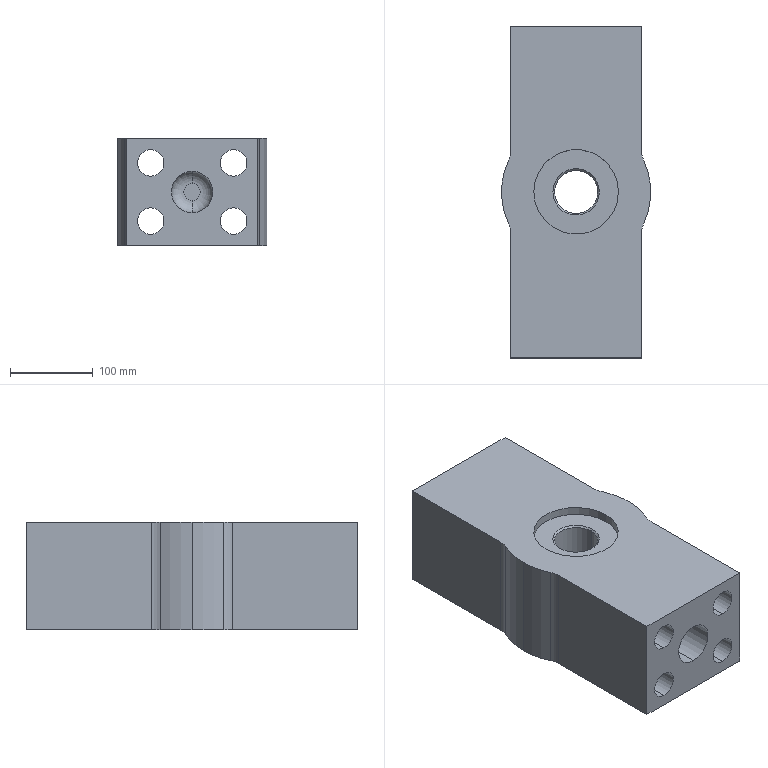Part | NX | features BREP 1 | 1 solid | 42 faces | box 180 x 400 x 130 mm | volume 6105398 mm3 | cylinder 23 | plane 11 | cone 4 | torus 4 | commonest cylinder face diameters 32 x8 50 x8 180 x3 52 x2 102 x2
STEP:
#1=CARTESIAN_POINT('',(50.,-200.,-51.));
#2=VERTEX_POINT('',#1);
#3=CARTESIAN_POINT('',(50.,-200.,-19.));
#4=VERTEX_POINT('',#3);
#5=CARTESIAN_POINT('',(50.,-200.,-35.));
#6=DIRECTION('',(0.,1.,0.));
#7=DIRECTION('',(0.,0.,-1.));
#8=AXIS2_PLACEMENT_3D('',#5,#6,#7);
#9=CIRCLE('',#8,16.);
#10=EDGE_CURVE('',#2,#4,#9,.T.);
#11=ORIENTED_EDGE('',*,*,#10,.F.);
#12=CARTESIAN_POINT('',(50.,200.,-51.));
#13=VERTEX_POINT('',#12);
#14=CARTESIAN_POINT('',(50.,-200.,-51.));
#15=DIRECTION('',(0.,1.,0.));
#16=VECTOR('',#15,1000.);
#17=LINE('',#14,#16);
#18=EDGE_CURVE('',#2,#13,#17,.T.);
#19=ORIENTED_EDGE('',*,*,#18,.T.);
#20=CARTESIAN_POINT('',(50.,200.,-19.));
#21=VERTEX_POINT('',#20);
#22=CARTESIAN_POINT('',(50.,200.,-35.));
#23=DIRECTION('',(0.,1.,0.));
#24=DIRECTION('',(0.,0.,-1.));
#25=AXIS2_PLACEMENT_3D('',#22,#23,#24);
#26=CIRCLE('',#25,16.);
#27=EDGE_CURVE('',#13,#21,#26,.T.);
#28=ORIENTED_EDGE('',*,*,#27,.T.);
#29=CARTESIAN_POINT('',(50.,-200.,-19.));
#30=DIRECTION('',(0.,1.,0.));
#31=VECTOR('',#30,1000.);
#32=LINE('',#29,#31);
#33=EDGE_CURVE('',#4,#21,#32,.T.);
#34=ORIENTED_EDGE('',*,*,#33,.F.);
#35=EDGE_LOOP('',(#11,#19,#28,#34));
#36=FACE_BOUND('',#35,.T.);
#37=CARTESIAN_POINT('',(50.,-200.,-35.));
#38=DIRECTION('',(0.,1.,0.));
#39=DIRECTION('',(0.,0.,-1.));
#40=AXIS2_PLACEMENT_3D('',#37,#38,#39);
#41=CYLINDRICAL_SURFACE('',#40,16.);
#42=ADVANCED_FACE('',(#36),#41,.F.);
#43=CARTESIAN_POINT('',(50.,-200.,19.));
#44=VERTEX_POINT('',#43);
#45=CARTESIAN_POINT('',(50.,-200.,51.));
#46=VERTEX_POINT('',#45);
#47=CARTESIAN_POINT('',(50.,-200.,35.));
#48=DIRECTION('',(0.,1.,0.));
#49=DIRECTION('',(0.,0.,1.));
#50=AXIS2_PLACEMENT_3D('',#47,#48,#49);
#51=CIRCLE('',#50,16.);
#52=EDGE_CURVE('',#44,#46,#51,.T.);
#53=ORIENTED_EDGE('',*,*,#52,.F.);
#54=CARTESIAN_POINT('',(50.,200.,19.));
#55=VERTEX_POINT('',#54);
#56=CARTESIAN_POINT('',(50.,-200.,19.));
#57=DIRECTION('',(0.,1.,0.));
#58=VECTOR('',#57,1000.);
#59=LINE('',#56,#58);
#60=EDGE_CURVE('',#44,#55,#59,.T.);
#61=ORIENTED_EDGE('',*,*,#60,.T.);
#62=CARTESIAN_POINT('',(50.,200.,51.));
#63=VERTEX_POINT('',#62);
#64=CARTESIAN_POINT('',(50.,200.,35.));
#65=DIRECTION('',(0.,1.,0.));
#66=DIRECTION('',(0.,0.,1.));
#67=AXIS2_PLACEMENT_3D('',#64,#65,#66);
#68=CIRCLE('',#67,16.);
#69=EDGE_CURVE('',#55,#63,#68,.T.);
#70=ORIENTED_EDGE('',*,*,#69,.T.);
#71=CARTESIAN_POINT('',(50.,-200.,51.));
#72=DIRECTION('',(0.,1.,0.));
#73=VECTOR('',#72,1000.);
#74=LINE('',#71,#73);
#75=EDGE_CURVE('',#46,#63,#74,.T.);
#76=ORIENTED_EDGE('',*,*,#75,.F.);
#77=EDGE_LOOP('',(#53,#61,#70,#76));
#78=FACE_BOUND('',#77,.T.);
#79=CARTESIAN_POINT('',(50.,-200.,35.));
#80=DIRECTION('',(0.,1.,0.));
#81=DIRECTION('',(0.,0.,-1.));
#82=AXIS2_PLACEMENT_3D('',#79,#80,#81);
#83=CYLINDRICAL_SURFACE('',#82,16.);
#84=ADVANCED_FACE('',(#78),#83,.F.);
#85=CARTESIAN_POINT('',(-50.,-200.,19.));
#86=VERTEX_POINT('',#85);
#87=CARTESIAN_POINT('',(-50.,-200.,51.));
#88=VERTEX_POINT('',#87);
#89=CARTESIAN_POINT('',(-50.,-200.,35.));
#90=DIRECTION('',(0.,1.,0.));
#91=DIRECTION('',(0.,0.,-1.));
#92=AXIS2_PLACEMENT_3D('',#89,#90,#91);
#93=CIRCLE('',#92,16.);
#94=EDGE_CURVE('',#86,#88,#93,.T.);
#95=ORIENTED_EDGE('',*,*,#94,.F.);
#96=CARTESIAN_POINT('',(-50.,200.,19.));
#97=VERTEX_POINT('',#96);
#98=CARTESIAN_POINT('',(-50.,-200.,19.));
#99=DIRECTION('',(0.,1.,0.));
#100=VECTOR('',#99,1000.);
#101=LINE('',#98,#100);
#102=EDGE_CURVE('',#86,#97,#101,.T.);
#103=ORIENTED_EDGE('',*,*,#102,.T.);
#104=CARTESIAN_POINT('',(-50.,200.,51.));
#105=VERTEX_POINT('',#104);
#106=CARTESIAN_POINT('',(-50.,200.,35.));
#107=DIRECTION('',(0.,1.,0.));
#108=DIRECTION('',(0.,0.,-1.));
#109=AXIS2_PLACEMENT_3D('',#106,#107,#108);
#110=CIRCLE('',#109,16.);
#111=EDGE_CURVE('',#97,#105,#110,.T.);
#112=ORIENTED_EDGE('',*,*,#111,.T.);
#113=CARTESIAN_POINT('',(-50.,-200.,51.));
#114=DIRECTION('',(0.,1.,0.));
#115=VECTOR('',#114,1000.);
#116=LINE('',#113,#115);
#117=EDGE_CURVE('',#88,#105,#116,.T.);
#118=ORIENTED_EDGE('',*,*,#117,.F.);
#119=EDGE_LOOP('',(#95,#103,#112,#118));
#120=FACE_BOUND('',#119,.T.);
#121=CARTESIAN_POINT('',(-50.,-200.,35.));
#122=DIRECTION('',(0.,1.,0.));
#123=DIRECTION('',(0.,0.,-1.));
#124=AXIS2_PLACEMENT_3D('',#121,#122,#123);
#125=CYLINDRICAL_SURFACE('',#124,16.);
#126=ADVANCED_FACE('',(#120),#125,.F.);
#127=CARTESIAN_POINT('',(-50.,-200.,-51.));
#128=VERTEX_POINT('',#127);
#129=CARTESIAN_POINT('',(-50.,-200.,-19.));
#130=VERTEX_POINT('',#129);
#131=CARTESIAN_POINT('',(-50.,-200.,-35.));
#132=DIRECTION('',(0.,1.,0.));
#133=DIRECTION('',(0.,0.,1.));
#134=AXIS2_PLACEMENT_3D('',#131,#132,#133);
#135=CIRCLE('',#134,16.);
#136=EDGE_CURVE('',#128,#130,#135,.T.);
#137=ORIENTED_EDGE('',*,*,#136,.F.);
#138=CARTESIAN_POINT('',(-50.,200.,-51.));
#139=VERTEX_POINT('',#138);
#140=CARTESIAN_POINT('',(-50.,-200.,-51.));
#141=DIRECTION('',(0.,1.,0.));
#142=VECTOR('',#141,1000.);
#143=LINE('',#140,#142);
#144=EDGE_CURVE('',#128,#139,#143,.T.);
#145=ORIENTED_EDGE('',*,*,#144,.T.);
#146=CARTESIAN_POINT('',(-50.,200.,-19.));
#147=VERTEX_POINT('',#146);
#148=CARTESIAN_POINT('',(-50.,200.,-35.));
#149=DIRECTION('',(0.,1.,0.));
#150=DIRECTION('',(0.,0.,1.));
#151=AXIS2_PLACEMENT_3D('',#148,#149,#150);
#152=CIRCLE('',#151,16.);
#153=EDGE_CURVE('',#139,#147,#152,.T.);
#154=ORIENTED_EDGE('',*,*,#153,.T.);
#155=CARTESIAN_POINT('',(-50.,-200.,-19.));
#156=DIRECTION('',(0.,1.,0.));
#157=VECTOR('',#156,1000.);
#158=LINE('',#155,#157);
#159=EDGE_CURVE('',#130,#147,#158,.T.);
#160=ORIENTED_EDGE('',*,*,#159,.F.);
#161=EDGE_LOOP('',(#137,#145,#154,#160));
#162=FACE_BOUND('',#161,.T.);
#163=CARTESIAN_POINT('',(-50.,-200.,-35.));
#164=DIRECTION('',(0.,1.,0.));
#165=DIRECTION('',(0.,0.,-1.));
#166=AXIS2_PLACEMENT_3D('',#163,#164,#165);
#167=CYLINDRICAL_SURFACE('',#166,16.);
#168=ADVANCED_FACE('',(#162),#167,.F.);
#169=CARTESIAN_POINT('',(26.,0.,-63.));
#170=VERTEX_POINT('',#169);
#171=CARTESIAN_POINT('',(-26.,0.,-63.));
#172=VERTEX_POINT('',#171);
#173=CARTESIAN_POINT('',(0.,0.,-63.));
#174=DIRECTION('',(0.,0.,-1.));
#175=DIRECTION('',(1.,0.,0.));
#176=AXIS2_PLACEMENT_3D('',#173,#174,#175);
#177=CIRCLE('',#176,26.);
#178=EDGE_CURVE('',#170,#172,#177,.T.);
#179=ORIENTED_EDGE('',*,*,#178,.F.);
#180=CARTESIAN_POINT('',(28.,0.,-65.));
#181=VERTEX_POINT('',#180);
#182=CARTESIAN_POINT('',(28.,0.,-65.));
#183=DIRECTION('',(0.7071,0.,-0.7071));
#184=VECTOR('',#183,1000.);
#185=LINE('',#182,#184);
#186=EDGE_CURVE('',#181,#170,#185,.F.);
#187=ORIENTED_EDGE('',*,*,#186,.F.);
#188=CARTESIAN_POINT('',(-28.,0.,-65.));
#189=VERTEX_POINT('',#188);
#190=CARTESIAN_POINT('',(0.,0.,-65.));
#191=DIRECTION('',(0.,0.,1.));
#192=DIRECTION('',(1.,0.,0.));
#193=AXIS2_PLACEMENT_3D('',#190,#191,#192);
#194=CIRCLE('',#193,28.);
#195=EDGE_CURVE('',#189,#181,#194,.T.);
#196=ORIENTED_EDGE('',*,*,#195,.F.);
#197=CARTESIAN_POINT('',(-28.,0.,-65.));
#198=DIRECTION('',(-0.7071,0.,-0.7071));
#199=VECTOR('',#198,1000.);
#200=LINE('',#197,#199);
#201=EDGE_CURVE('',#189,#172,#200,.F.);
#202=ORIENTED_EDGE('',*,*,#201,.T.);
#203=EDGE_LOOP('',(#179,#187,#196,#202));
#204=FACE_BOUND('',#203,.T.);
#205=CARTESIAN_POINT('',(0.,0.,-65.));
#206=DIRECTION('',(0.,0.,-1.));
#207=DIRECTION('',(1.,0.,0.));
#208=AXIS2_PLACEMENT_3D('',#205,#206,#207);
#209=CONICAL_SURFACE('',#208,28.,0.7854);
#210=ADVANCED_FACE('',(#204),#209,.F.);
#211=CARTESIAN_POINT('',(-26.,0.,53.));
#212=VERTEX_POINT('',#211);
#213=CARTESIAN_POINT('',(26.,0.,53.));
#214=VERTEX_POINT('',#213);
#215=CARTESIAN_POINT('',(0.,0.,53.));
#216=DIRECTION('',(0.,0.,1.));
#217=DIRECTION('',(1.,0.,0.));
#218=AXIS2_PLACEMENT_3D('',#215,#216,#217);
#219=CIRCLE('',#218,26.);
#220=EDGE_CURVE('',#212,#214,#219,.T.);
#221=ORIENTED_EDGE('',*,*,#220,.F.);
#222=CARTESIAN_POINT('',(-28.,0.,55.));
#223=VERTEX_POINT('',#222);
#224=CARTESIAN_POINT('',(-26.,0.,53.));
#225=DIRECTION('',(-0.7071,0.,0.7071));
#226=VECTOR('',#225,1000.);
#227=LINE('',#224,#226);
#228=EDGE_CURVE('',#212,#223,#227,.T.);
#229=ORIENTED_EDGE('',*,*,#228,.T.);
#230=CARTESIAN_POINT('',(28.,0.,55.));
#231=VERTEX_POINT('',#230);
#232=CARTESIAN_POINT('',(0.,0.,55.));
#233=DIRECTION('',(0.,0.,-1.));
#234=DIRECTION('',(1.,0.,0.));
#235=AXIS2_PLACEMENT_3D('',#232,#233,#234);
#236=CIRCLE('',#235,28.);
#237=EDGE_CURVE('',#231,#223,#236,.T.);
#238=ORIENTED_EDGE('',*,*,#237,.F.);
#239=CARTESIAN_POINT('',(26.,0.,53.));
#240=DIRECTION('',(0.7071,0.,0.7071));
#241=VECTOR('',#240,1000.);
#242=LINE('',#239,#241);
#243=EDGE_CURVE('',#214,#231,#242,.T.);
#244=ORIENTED_EDGE('',*,*,#243,.F.);
#245=EDGE_LOOP('',(#221,#229,#238,#244));
#246=FACE_BOUND('',#245,.T.);
#247=CARTESIAN_POINT('',(0.,0.,53.));
#248=DIRECTION('',(0.,0.,1.));
#249=DIRECTION('',(-1.,0.,0.));
#250=AXIS2_PLACEMENT_3D('',#247,#248,#249);
#251=CONICAL_SURFACE('',#250,26.,0.7854);
#252=ADVANCED_FACE('',(#246),#251,.F.);
#253=CARTESIAN_POINT('',(0.,-45.,-25.));
#254=VERTEX_POINT('',#253);
#255=CARTESIAN_POINT('',(0.,-45.,25.));
#256=VERTEX_POINT('',#255);
#257=CARTESIAN_POINT('',(0.,-45.,0.));
#258=DIRECTION('',(0.,-1.,0.));
#259=DIRECTION('',(0.,0.,-1.));
#260=AXIS2_PLACEMENT_3D('',#257,#258,#259);
#261=CIRCLE('',#260,25.);
#262=EDGE_CURVE('',#254,#256,#261,.T.);
#263=ORIENTED_EDGE('',*,*,#262,.T.);
#264=CARTESIAN_POINT('',(0.,-30.,10.));
#265=VERTEX_POINT('',#264);
#266=CARTESIAN_POINT('',(0.,-45.,10.));
#267=DIRECTION('',(-1.,0.,0.));
#268=DIRECTION('',(0.,0.,1.));
#269=AXIS2_PLACEMENT_3D('',#266,#267,#268);
#270=CIRCLE('',#269,15.);
#271=EDGE_CURVE('',#265,#256,#270,.F.);
#272=ORIENTED_EDGE('',*,*,#271,.F.);
#273=CARTESIAN_POINT('',(0.,-30.,-10.));
#274=VERTEX_POINT('',#273);
#275=CARTESIAN_POINT('',(0.,-30.,0.));
#276=DIRECTION('',(0.,-1.,0.));
#277=DIRECTION('',(0.,0.,-1.));
#278=AXIS2_PLACEMENT_3D('',#275,#276,#277);
#279=CIRCLE('',#278,10.);
#280=EDGE_CURVE('',#274,#265,#279,.T.);
#281=ORIENTED_EDGE('',*,*,#280,.F.);
#282=CARTESIAN_POINT('',(0.,-45.,-10.));
#283=DIRECTION('',(1.,0.,0.));
#284=DIRECTION('',(0.,0.,-1.));
#285=AXIS2_PLACEMENT_3D('',#282,#283,#284);
#286=CIRCLE('',#285,15.);
#287=EDGE_CURVE('',#274,#254,#286,.F.);
#288=ORIENTED_EDGE('',*,*,#287,.T.);
#289=EDGE_LOOP('',(#263,#272,#281,#288));
#290=FACE_BOUND('',#289,.T.);
#291=CARTESIAN_POINT('',(0.,-45.,0.));
#292=DIRECTION('',(0.,1.,0.));
#293=DIRECTION('',(0.,0.,1.));
#294=AXIS2_PLACEMENT_3D('',#291,#292,#293);
#295=DEGENERATE_TOROIDAL_SURFACE('',#294,10.,15.,.T.);
#296=ADVANCED_FACE('',(#290),#295,.F.);
#297=CARTESIAN_POINT('',(0.,-200.,-25.));
#298=VERTEX_POINT('',#297);
#299=CARTESIAN_POINT('',(0.,-200.,25.));
#300=VERTEX_POINT('',#299);
#301=CARTESIAN_POINT('',(0.,-200.,0.));
#302=DIRECTION('',(0.,-1.,0.));
#303=DIRECTION('',(0.,0.,-1.));
#304=AXIS2_PLACEMENT_3D('',#301,#302,#303);
#305=CIRCLE('',#304,25.);
#306=EDGE_CURVE('',#298,#300,#305,.T.);
#307=ORIENTED_EDGE('',*,*,#306,.T.);
#308=CARTESIAN_POINT('',(0.,0.,25.));
#309=DIRECTION('',(0.,1.,0.));
#310=VECTOR('',#309,1000.);
#311=LINE('',#308,#310);
#312=EDGE_CURVE('',#256,#300,#311,.F.);
#313=ORIENTED_EDGE('',*,*,#312,.F.);
#314=ORIENTED_EDGE('',*,*,#262,.F.);
#315=CARTESIAN_POINT('',(0.,0.,-25.));
#316=DIRECTION('',(0.,1.,0.));
#317=VECTOR('',#316,1000.);
#318=LINE('',#315,#317);
#319=EDGE_CURVE('',#254,#298,#318,.F.);
#320=ORIENTED_EDGE('',*,*,#319,.T.);
#321=EDGE_LOOP('',(#307,#313,#314,#320));
#322=FACE_BOUND('',#321,.T.);
#323=CARTESIAN_POINT('',(0.,0.,0.));
#324=DIRECTION('',(0.,1.,0.));
#325=DIRECTION('',(0.,0.,1.));
#326=AXIS2_PLACEMENT_3D('',#323,#324,#325);
#327=CYLINDRICAL_SURFACE('',#326,25.);
#328=ADVANCED_FACE('',(#322),#327,.F.);
#329=CARTESIAN_POINT('',(0.,45.,25.));
#330=VERTEX_POINT('',#329);
#331=CARTESIAN_POINT('',(0.,45.,-25.));
#332=VERTEX_POINT('',#331);
#333=CARTESIAN_POINT('',(0.,45.,0.));
#334=DIRECTION('',(0.,-1.,0.));
#335=DIRECTION('',(0.,0.,-1.));
#336=AXIS2_PLACEMENT_3D('',#333,#334,#335);
#337=CIRCLE('',#336,25.);
#338=EDGE_CURVE('',#330,#332,#337,.T.);
#339=ORIENTED_EDGE('',*,*,#338,.F.);
#340=CARTESIAN_POINT('',(0.,30.,10.));
#341=VERTEX_POINT('',#340);
#342=CARTESIAN_POINT('',(0.,45.,10.));
#343=DIRECTION('',(1.,0.,0.));
#344=DIRECTION('',(0.,0.,-1.));
#345=AXIS2_PLACEMENT_3D('',#342,#343,#344);
#346=CIRCLE('',#345,15.);
#347=EDGE_CURVE('',#341,#330,#346,.F.);
#348=ORIENTED_EDGE('',*,*,#347,.F.);
#349=CARTESIAN_POINT('',(0.,30.,-10.));
#350=VERTEX_POINT('',#349);
#351=CARTESIAN_POINT('',(0.,30.,0.));
#352=DIRECTION('',(0.,-1.,0.));
#353=DIRECTION('',(0.,0.,-1.));
#354=AXIS2_PLACEMENT_3D('',#351,#352,#353);
#355=CIRCLE('',#354,10.);
#356=EDGE_CURVE('',#341,#350,#355,.T.);
#357=ORIENTED_EDGE('',*,*,#356,.T.);
#358=CARTESIAN_POINT('',(0.,45.,-10.));
#359=DIRECTION('',(-1.,0.,0.));
#360=DIRECTION('',(0.,0.,1.));
#361=AXIS2_PLACEMENT_3D('',#358,#359,#360);
#362=CIRCLE('',#361,15.);
#363=EDGE_CURVE('',#350,#332,#362,.F.);
#364=ORIENTED_EDGE('',*,*,#363,.T.);
#365=EDGE_LOOP('',(#339,#348,#357,#364));
#366=FACE_BOUND('',#365,.T.);
#367=CARTESIAN_POINT('',(0.,45.,0.));
#368=DIRECTION('',(0.,-1.,0.));
#369=DIRECTION('',(0.,0.,1.));
#370=AXIS2_PLACEMENT_3D('',#367,#368,#369);
#371=DEGENERATE_TOROIDAL_SURFACE('',#370,10.,15.,.T.);
#372=ADVANCED_FACE('',(#366),#371,.F.);
#373=CARTESIAN_POINT('',(0.,200.,25.));
#374=VERTEX_POINT('',#373);
#375=CARTESIAN_POINT('',(0.,200.,-25.));
#376=VERTEX_POINT('',#375);
#377=CARTESIAN_POINT('',(0.,200.,0.));
#378=DIRECTION('',(0.,-1.,0.));
#379=DIRECTION('',(0.,0.,-1.));
#380=AXIS2_PLACEMENT_3D('',#377,#378,#379);
#381=CIRCLE('',#380,25.);
#382=EDGE_CURVE('',#374,#376,#381,.T.);
#383=ORIENTED_EDGE('',*,*,#382,.F.);
#384=CARTESIAN_POINT('',(0.,0.,25.));
#385=DIRECTION('',(0.,-1.,0.));
#386=VECTOR('',#385,1000.);
#387=LINE('',#384,#386);
#388=EDGE_CURVE('',#330,#374,#387,.F.);
#389=ORIENTED_EDGE('',*,*,#388,.F.);
#390=ORIENTED_EDGE('',*,*,#338,.T.);
#391=CARTESIAN_POINT('',(0.,0.,-25.));
#392=DIRECTION('',(0.,-1.,0.));
#393=VECTOR('',#392,1000.);
#394=LINE('',#391,#393);
#395=EDGE_CURVE('',#332,#376,#394,.F.);
#396=ORIENTED_EDGE('',*,*,#395,.T.);
#397=EDGE_LOOP('',(#383,#389,#390,#396));
#398=FACE_BOUND('',#397,.T.);
#399=CARTESIAN_POINT('',(0.,0.,0.));
#400=DIRECTION('',(0.,-1.,0.));
#401=DIRECTION('',(0.,0.,1.));
#402=AXIS2_PLACEMENT_3D('',#399,#400,#401);
#403=CYLINDRICAL_SURFACE('',#402,25.);
#404=ADVANCED_FACE('',(#398),#403,.F.);
#405=CARTESIAN_POINT('',(-51.,0.,55.));
#406=VERTEX_POINT('',#405);
#407=CARTESIAN_POINT('',(51.,0.,55.));
#408=VERTEX_POINT('',#407);
#409=CARTESIAN_POINT('',(0.,0.,55.));
#410=DIRECTION('',(0.,0.,1.));
#411=DIRECTION('',(1.,0.,0.));
#412=AXIS2_PLACEMENT_3D('',#409,#410,#411);
#413=CIRCLE('',#412,51.);
#414=EDGE_CURVE('',#406,#408,#413,.T.);
#415=ORIENTED_EDGE('',*,*,#414,.F.);
#416=CARTESIAN_POINT('',(-51.,0.,65.));
#417=VERTEX_POINT('',#416);
#418=CARTESIAN_POINT('',(-51.,0.,55.));
#419=DIRECTION('',(0.,0.,1.));
#420=VECTOR('',#419,1000.);
#421=LINE('',#418,#420);
#422=EDGE_CURVE('',#406,#417,#421,.T.);
#423=ORIENTED_EDGE('',*,*,#422,.T.);
#424=CARTESIAN_POINT('',(51.,0.,65.));
#425=VERTEX_POINT('',#424);
#426=CARTESIAN_POINT('',(0.,0.,65.));
#427=DIRECTION('',(0.,0.,1.));
#428=DIRECTION('',(1.,0.,0.));
#429=AXIS2_PLACEMENT_3D('',#426,#427,#428);
#430=CIRCLE('',#429,51.);
#431=EDGE_CURVE('',#417,#425,#430,.T.);
#432=ORIENTED_EDGE('',*,*,#431,.T.);
#433=CARTESIAN_POINT('',(51.,0.,55.));
#434=DIRECTION('',(0.,0.,1.));
#435=VECTOR('',#434,1000.);
#436=LINE('',#433,#435);
#437=EDGE_CURVE('',#408,#425,#436,.T.);
#438=ORIENTED_EDGE('',*,*,#437,.F.);
#439=EDGE_LOOP('',(#415,#423,#432,#438));
#440=FACE_BOUND('',#439,.T.);
#441=CARTESIAN_POINT('',(0.,0.,55.));
#442=DIRECTION('',(0.,0.,1.));
#443=DIRECTION('',(-1.,0.,0.));
#444=AXIS2_PLACEMENT_3D('',#441,#442,#443);
#445=CYLINDRICAL_SURFACE('',#444,51.);
#446=ADVANCED_FACE('',(#440),#445,.F.);
#447=CARTESIAN_POINT('',(-90.,0.,65.));
#448=VERTEX_POINT('',#447);
#449=CARTESIAN_POINT('',(-81.391,-38.412,65.));
#450=VERTEX_POINT('',#449);
#451=CARTESIAN_POINT('',(0.,0.,65.));
#452=DIRECTION('',(0.,0.,1.));
#453=DIRECTION('',(1.,0.,0.));
#454=AXIS2_PLACEMENT_3D('',#451,#452,#453);
#455=CIRCLE('',#454,90.);
#456=EDGE_CURVE('',#448,#450,#455,.T.);
#457=ORIENTED_EDGE('',*,*,#456,.F.);
#458=CARTESIAN_POINT('',(-90.,0.,-65.));
#459=VERTEX_POINT('',#458);
#460=CARTESIAN_POINT('',(-90.,0.,65.));
#461=DIRECTION('',(0.,0.,-1.));
#462=VECTOR('',#461,1000.);
#463=LINE('',#460,#462);
#464=EDGE_CURVE('',#448,#459,#463,.T.);
#465=ORIENTED_EDGE('',*,*,#464,.T.);
#466=CARTESIAN_POINT('',(-81.391,-38.412,-65.));
#467=VERTEX_POINT('',#466);
#468=CARTESIAN_POINT('',(0.,0.,-65.));
#469=DIRECTION('',(0.,0.,1.));
#470=DIRECTION('',(1.,0.,0.));
#471=AXIS2_PLACEMENT_3D('',#468,#469,#470);
#472=CIRCLE('',#471,90.);
#473=EDGE_CURVE('',#459,#467,#472,.T.);
#474=ORIENTED_EDGE('',*,*,#473,.T.);
#475=CARTESIAN_POINT('',(-81.391,-38.412,65.));
#476=DIRECTION('',(0.,0.,-1.));
#477=VECTOR('',#476,1000.);
#478=LINE('',#475,#477);
#479=EDGE_CURVE('',#450,#467,#478,.T.);
#480=ORIENTED_EDGE('',*,*,#479,.F.);
#481=EDGE_LOOP('',(#457,#465,#474,#480));
#482=FACE_BOUND('',#481,.T.);
#483=CARTESIAN_POINT('',(0.,0.,65.));
#484=DIRECTION('',(0.,0.,-1.));
#485=DIRECTION('',(1.,0.,0.));
#486=AXIS2_PLACEMENT_3D('',#483,#484,#485);
#487=CYLINDRICAL_SURFACE('',#486,90.);
#488=ADVANCED_FACE('',(#482),#487,.T.);
#489=ORIENTED_EDGE('',*,*,#220,.T.);
#490=CARTESIAN_POINT('',(26.,0.,65.));
#491=DIRECTION('',(0.,0.,-1.));
#492=VECTOR('',#491,1000.);
#493=LINE('',#490,#492);
#494=EDGE_CURVE('',#170,#214,#493,.F.);
#495=ORIENTED_EDGE('',*,*,#494,.F.);
#496=ORIENTED_EDGE('',*,*,#178,.T.);
#497=CARTESIAN_POINT('',(-26.,0.,65.));
#498=DIRECTION('',(0.,0.,-1.));
#499=VECTOR('',#498,1000.);
#500=LINE('',#497,#499);
#501=EDGE_CURVE('',#172,#212,#500,.F.);
#502=ORIENTED_EDGE('',*,*,#501,.T.);
#503=EDGE_LOOP('',(#489,#495,#496,#502));
#504=FACE_BOUND('',#503,.T.);
#505=CARTESIAN_POINT('',(0.,0.,65.));
#506=DIRECTION('',(0.,0.,-1.));
#507=DIRECTION('',(1.,0.,0.));
#508=AXIS2_PLACEMENT_3D('',#505,#506,#507);
#509=CYLINDRICAL_SURFACE('',#508,26.);
#510=ADVANCED_FACE('',(#504),#509,.F.);
#511=CARTESIAN_POINT('',(50.,-200.,-35.));
#512=DIRECTION('',(0.,1.,0.));
#513=DIRECTION('',(0.,0.,-1.));
#514=AXIS2_PLACEMENT_3D('',#511,#512,#513);
#515=CIRCLE('',#514,16.);
#516=EDGE_CURVE('',#4,#2,#515,.T.);
#517=ORIENTED_EDGE('',*,*,#516,.T.);
#518=ORIENTED_EDGE('',*,*,#10,.T.);
#519=EDGE_LOOP('',(#517,#518));
#520=FACE_BOUND('',#519,.T.);
#521=CARTESIAN_POINT('',(50.,-200.,35.));
#522=DIRECTION('',(0.,1.,0.));
#523=DIRECTION('',(0.,0.,1.));
#524=AXIS2_PLACEMENT_3D('',#521,#522,#523);
#525=CIRCLE('',#524,16.);
#526=EDGE_CURVE('',#46,#44,#525,.T.);
#527=ORIENTED_EDGE('',*,*,#526,.T.);
#528=ORIENTED_EDGE('',*,*,#52,.T.);
#529=EDGE_LOOP('',(#527,#528));
#530=FACE_BOUND('',#529,.T.);
#531=CARTESIAN_POINT('',(-50.,-200.,35.));
#532=DIRECTION('',(0.,1.,0.));
#533=DIRECTION('',(0.,0.,-1.));
#534=AXIS2_PLACEMENT_3D('',#531,#532,#533);
#535=CIRCLE('',#534,16.);
#536=EDGE_CURVE('',#88,#86,#535,.T.);
#537=ORIENTED_EDGE('',*,*,#536,.T.);
#538=ORIENTED_EDGE('',*,*,#94,.T.);
#539=EDGE_LOOP('',(#537,#538));
#540=FACE_BOUND('',#539,.T.);
#541=CARTESIAN_POINT('',(-50.,-200.,-35.));
#542=DIRECTION('',(0.,1.,0.));
#543=DIRECTION('',(0.,0.,1.));
#544=AXIS2_PLACEMENT_3D('',#541,#542,#543);
#545=CIRCLE('',#544,16.);
#546=EDGE_CURVE('',#130,#128,#545,.T.);
#547=ORIENTED_EDGE('',*,*,#546,.T.);
#548=ORIENTED_EDGE('',*,*,#136,.T.);
#549=EDGE_LOOP('',(#547,#548));
#550=FACE_BOUND('',#549,.T.);
#551=CARTESIAN_POINT('',(-79.,-200.,-65.));
#552=VERTEX_POINT('',#551);
#553=CARTESIAN_POINT('',(79.,-200.,-65.));
#554=VERTEX_POINT('',#553);
#555=CARTESIAN_POINT('',(-79.,-200.,-65.));
#556=DIRECTION('',(1.,0.,0.));
#557=VECTOR('',#556,1000.);
#558=LINE('',#555,#557);
#559=EDGE_CURVE('',#552,#554,#558,.T.);
#560=ORIENTED_EDGE('',*,*,#559,.T.);
#561=CARTESIAN_POINT('',(79.,-200.,65.));
#562=VERTEX_POINT('',#561);
#563=CARTESIAN_POINT('',(79.,-200.,65.));
#564=DIRECTION('',(0.,0.,-1.));
#565=VECTOR('',#564,1000.);
#566=LINE('',#563,#565);
#567=EDGE_CURVE('',#562,#554,#566,.T.);
#568=ORIENTED_EDGE('',*,*,#567,.F.);
#569=CARTESIAN_POINT('',(-79.,-200.,65.));
#570=VERTEX_POINT('',#569);
#571=CARTESIAN_POINT('',(-79.,-200.,65.));
#572=DIRECTION('',(1.,0.,0.));
#573=VECTOR('',#572,1000.);
#574=LINE('',#571,#573);
#575=EDGE_CURVE('',#570,#562,#574,.T.);
#576=ORIENTED_EDGE('',*,*,#575,.F.);
#577=CARTESIAN_POINT('',(-79.,-200.,65.));
#578=DIRECTION('',(0.,0.,-1.));
#579=VECTOR('',#578,1000.);
#580=LINE('',#577,#579);
#581=EDGE_CURVE('',#570,#552,#580,.T.);
#582=ORIENTED_EDGE('',*,*,#581,.T.);
#583=EDGE_LOOP('',(#560,#568,#576,#582));
#584=FACE_BOUND('',#583,.T.);
#585=ORIENTED_EDGE('',*,*,#306,.F.);
#586=CARTESIAN_POINT('',(0.,-200.,0.));
#587=DIRECTION('',(0.,-1.,0.));
#588=DIRECTION('',(0.,0.,-1.));
#589=AXIS2_PLACEMENT_3D('',#586,#587,#588);
#590=CIRCLE('',#589,25.);
#591=EDGE_CURVE('',#300,#298,#590,.T.);
#592=ORIENTED_EDGE('',*,*,#591,.F.);
#593=EDGE_LOOP('',(#585,#592));
#594=FACE_BOUND('',#593,.T.);
#595=CARTESIAN_POINT('',(-79.,-200.,65.));
#596=DIRECTION('',(0.,1.,0.));
#597=DIRECTION('',(0.,0.,-1.));
#598=AXIS2_PLACEMENT_3D('',#595,#596,#597);
#599=PLANE('',#598);
#600=ADVANCED_FACE('',(#520,#530,#540,#550,#584,#594),#599,.F.);
#601=CARTESIAN_POINT('',(50.,200.,-35.));
#602=DIRECTION('',(0.,1.,0.));
#603=DIRECTION('',(0.,0.,-1.));
#604=AXIS2_PLACEMENT_3D('',#601,#602,#603);
#605=CIRCLE('',#604,16.);
#606=EDGE_CURVE('',#21,#13,#605,.T.);
#607=ORIENTED_EDGE('',*,*,#606,.F.);
#608=ORIENTED_EDGE('',*,*,#27,.F.);
#609=EDGE_LOOP('',(#607,#608));
#610=FACE_BOUND('',#609,.T.);
#611=CARTESIAN_POINT('',(50.,200.,35.));
#612=DIRECTION('',(0.,1.,0.));
#613=DIRECTION('',(0.,0.,1.));
#614=AXIS2_PLACEMENT_3D('',#611,#612,#613);
#615=CIRCLE('',#614,16.);
#616=EDGE_CURVE('',#63,#55,#615,.T.);
#617=ORIENTED_EDGE('',*,*,#616,.F.);
#618=ORIENTED_EDGE('',*,*,#69,.F.);
#619=EDGE_LOOP('',(#617,#618));
#620=FACE_BOUND('',#619,.T.);
#621=CARTESIAN_POINT('',(-50.,200.,35.));
#622=DIRECTION('',(0.,1.,0.));
#623=DIRECTION('',(0.,0.,-1.));
#624=AXIS2_PLACEMENT_3D('',#621,#622,#623);
#625=CIRCLE('',#624,16.);
#626=EDGE_CURVE('',#105,#97,#625,.T.);
#627=ORIENTED_EDGE('',*,*,#626,.F.);
#628=ORIENTED_EDGE('',*,*,#111,.F.);
#629=EDGE_LOOP('',(#627,#628));
#630=FACE_BOUND('',#629,.T.);
#631=CARTESIAN_POINT('',(-50.,200.,-35.));
#632=DIRECTION('',(0.,1.,0.));
#633=DIRECTION('',(0.,0.,1.));
#634=AXIS2_PLACEMENT_3D('',#631,#632,#633);
#635=CIRCLE('',#634,16.);
#636=EDGE_CURVE('',#147,#139,#635,.T.);
#637=ORIENTED_EDGE('',*,*,#636,.F.);
#638=ORIENTED_EDGE('',*,*,#153,.F.);
#639=EDGE_LOOP('',(#637,#638));
#640=FACE_BOUND('',#639,.T.);
#641=CARTESIAN_POINT('',(79.,200.,-65.));
#642=VERTEX_POINT('',#641);
#643=CARTESIAN_POINT('',(-79.,200.,-65.));
#644=VERTEX_POINT('',#643);
#645=CARTESIAN_POINT('',(-79.,200.,-65.));
#646=DIRECTION('',(-1.,0.,0.));
#647=VECTOR('',#646,1000.);
#648=LINE('',#645,#647);
#649=EDGE_CURVE('',#642,#644,#648,.T.);
#650=ORIENTED_EDGE('',*,*,#649,.T.);
#651=CARTESIAN_POINT('',(-79.,200.,65.));
#652=VERTEX_POINT('',#651);
#653=CARTESIAN_POINT('',(-79.,200.,65.));
#654=DIRECTION('',(0.,0.,-1.));
#655=VECTOR('',#654,1000.);
#656=LINE('',#653,#655);
#657=EDGE_CURVE('',#652,#644,#656,.T.);
#658=ORIENTED_EDGE('',*,*,#657,.F.);
#659=CARTESIAN_POINT('',(79.,200.,65.));
#660=VERTEX_POINT('',#659);
#661=CARTESIAN_POINT('',(-79.,200.,65.));
#662=DIRECTION('',(-1.,0.,0.));
#663=VECTOR('',#662,1000.);
#664=LINE('',#661,#663);
#665=EDGE_CURVE('',#660,#652,#664,.T.);
#666=ORIENTED_EDGE('',*,*,#665,.F.);
#667=CARTESIAN_POINT('',(79.,200.,65.));
#668=DIRECTION('',(0.,0.,-1.));
#669=VECTOR('',#668,1000.);
#670=LINE('',#667,#669);
#671=EDGE_CURVE('',#660,#642,#670,.T.);
#672=ORIENTED_EDGE('',*,*,#671,.T.);
#673=EDGE_LOOP('',(#650,#658,#666,#672));
#674=FACE_BOUND('',#673,.T.);
#675=CARTESIAN_POINT('',(0.,200.,0.));
#676=DIRECTION('',(0.,-1.,0.));
#677=DIRECTION('',(0.,0.,-1.));
#678=AXIS2_PLACEMENT_3D('',#675,#676,#677);
#679=CIRCLE('',#678,25.);
#680=EDGE_CURVE('',#376,#374,#679,.T.);
#681=ORIENTED_EDGE('',*,*,#680,.T.);
#682=ORIENTED_EDGE('',*,*,#382,.T.);
#683=EDGE_LOOP('',(#681,#682));
#684=FACE_BOUND('',#683,.T.);
#685=CARTESIAN_POINT('',(-79.,200.,65.));
#686=DIRECTION('',(0.,-1.,0.));
#687=DIRECTION('',(0.,0.,1.));
#688=AXIS2_PLACEMENT_3D('',#685,#686,#687);
#689=PLANE('',#688);
#690=ADVANCED_FACE('',(#610,#620,#630,#640,#674,#684),#689,.F.);
#691=ORIENTED_EDGE('',*,*,#494,.T.);
#692=CARTESIAN_POINT('',(0.,0.,53.));
#693=DIRECTION('',(0.,0.,1.));
#694=DIRECTION('',(1.,0.,0.));
#695=AXIS2_PLACEMENT_3D('',#692,#693,#694);
#696=CIRCLE('',#695,26.);
#697=EDGE_CURVE('',#214,#212,#696,.T.);
#698=ORIENTED_EDGE('',*,*,#697,.T.);
#699=ORIENTED_EDGE('',*,*,#501,.F.);
#700=CARTESIAN_POINT('',(0.,0.,-63.));
#701=DIRECTION('',(0.,0.,-1.));
#702=DIRECTION('',(1.,0.,0.));
#703=AXIS2_PLACEMENT_3D('',#700,#701,#702);
#704=CIRCLE('',#703,26.);
#705=EDGE_CURVE('',#172,#170,#704,.T.);
#706=ORIENTED_EDGE('',*,*,#705,.T.);
#707=EDGE_LOOP('',(#691,#698,#699,#706));
#708=FACE_BOUND('',#707,.T.);
#709=CARTESIAN_POINT('',(0.,0.,65.));
#710=DIRECTION('',(0.,0.,-1.));
#711=DIRECTION('',(1.,0.,0.));
#712=AXIS2_PLACEMENT_3D('',#709,#710,#711);
#713=CYLINDRICAL_SURFACE('',#712,26.);
#714=ADVANCED_FACE('',(#708),#713,.F.);
#715=CARTESIAN_POINT('',(0.,0.,65.));
#716=DIRECTION('',(0.,0.,1.));
#717=DIRECTION('',(1.,0.,0.));
#718=AXIS2_PLACEMENT_3D('',#715,#716,#717);
#719=CIRCLE('',#718,51.);
#720=EDGE_CURVE('',#425,#417,#719,.T.);
#721=ORIENTED_EDGE('',*,*,#720,.F.);
#722=ORIENTED_EDGE('',*,*,#431,.F.);
#723=EDGE_LOOP('',(#721,#722));
#724=FACE_BOUND('',#723,.T.);
#725=CARTESIAN_POINT('',(81.391,38.412,65.));
#726=VERTEX_POINT('',#725);
#727=CARTESIAN_POINT('',(79.,49.082,65.));
#728=VERTEX_POINT('',#727);
#729=CARTESIAN_POINT('',(104.,49.082,65.));
#730=DIRECTION('',(0.,0.,-1.));
#731=DIRECTION('',(1.,0.,0.));
#732=AXIS2_PLACEMENT_3D('',#729,#730,#731);
#733=CIRCLE('',#732,25.);
#734=EDGE_CURVE('',#726,#728,#733,.T.);
#735=ORIENTED_EDGE('',*,*,#734,.T.);
#736=CARTESIAN_POINT('',(79.,200.,65.));
#737=DIRECTION('',(0.,1.,0.));
#738=VECTOR('',#737,1000.);
#739=LINE('',#736,#738);
#740=EDGE_CURVE('',#728,#660,#739,.T.);
#741=ORIENTED_EDGE('',*,*,#740,.T.);
#742=ORIENTED_EDGE('',*,*,#665,.T.);
#743=CARTESIAN_POINT('',(-79.,49.082,65.));
#744=VERTEX_POINT('',#743);
#745=CARTESIAN_POINT('',(-79.,200.,65.));
#746=DIRECTION('',(0.,-1.,0.));
#747=VECTOR('',#746,1000.);
#748=LINE('',#745,#747);
#749=EDGE_CURVE('',#652,#744,#748,.T.);
#750=ORIENTED_EDGE('',*,*,#749,.T.);
#751=CARTESIAN_POINT('',(-81.391,38.412,65.));
#752=VERTEX_POINT('',#751);
#753=CARTESIAN_POINT('',(-104.,49.082,65.));
#754=DIRECTION('',(0.,0.,-1.));
#755=DIRECTION('',(-1.,0.,0.));
#756=AXIS2_PLACEMENT_3D('',#753,#754,#755);
#757=CIRCLE('',#756,25.);
#758=EDGE_CURVE('',#744,#752,#757,.T.);
#759=ORIENTED_EDGE('',*,*,#758,.T.);
#760=CARTESIAN_POINT('',(0.,0.,65.));
#761=DIRECTION('',(0.,0.,1.));
#762=DIRECTION('',(1.,0.,0.));
#763=AXIS2_PLACEMENT_3D('',#760,#761,#762);
#764=CIRCLE('',#763,90.);
#765=EDGE_CURVE('',#752,#448,#764,.T.);
#766=ORIENTED_EDGE('',*,*,#765,.T.);
#767=ORIENTED_EDGE('',*,*,#456,.T.);
#768=CARTESIAN_POINT('',(-79.,-49.082,65.));
#769=VERTEX_POINT('',#768);
#770=CARTESIAN_POINT('',(-104.,-49.082,65.));
#771=DIRECTION('',(0.,0.,-1.));
#772=DIRECTION('',(-1.,0.,0.));
#773=AXIS2_PLACEMENT_3D('',#770,#771,#772);
#774=CIRCLE('',#773,25.);
#775=EDGE_CURVE('',#450,#769,#774,.T.);
#776=ORIENTED_EDGE('',*,*,#775,.T.);
#777=CARTESIAN_POINT('',(-79.,-200.,65.));
#778=DIRECTION('',(0.,-1.,0.));
#779=VECTOR('',#778,1000.);
#780=LINE('',#777,#779);
#781=EDGE_CURVE('',#769,#570,#780,.T.);
#782=ORIENTED_EDGE('',*,*,#781,.T.);
#783=ORIENTED_EDGE('',*,*,#575,.T.);
#784=CARTESIAN_POINT('',(79.,-49.082,65.));
#785=VERTEX_POINT('',#784);
#786=CARTESIAN_POINT('',(79.,-200.,65.));
#787=DIRECTION('',(0.,1.,0.));
#788=VECTOR('',#787,1000.);
#789=LINE('',#786,#788);
#790=EDGE_CURVE('',#562,#785,#789,.T.);
#791=ORIENTED_EDGE('',*,*,#790,.T.);
#792=CARTESIAN_POINT('',(81.391,-38.412,65.));
#793=VERTEX_POINT('',#792);
#794=CARTESIAN_POINT('',(104.,-49.082,65.));
#795=DIRECTION('',(0.,0.,-1.));
#796=DIRECTION('',(-1.,0.,0.));
#797=AXIS2_PLACEMENT_3D('',#794,#795,#796);
#798=CIRCLE('',#797,25.);
#799=EDGE_CURVE('',#785,#793,#798,.T.);
#800=ORIENTED_EDGE('',*,*,#799,.T.);
#801=CARTESIAN_POINT('',(0.,0.,65.));
#802=DIRECTION('',(0.,0.,1.));
#803=DIRECTION('',(1.,0.,0.));
#804=AXIS2_PLACEMENT_3D('',#801,#802,#803);
#805=CIRCLE('',#804,90.);
#806=EDGE_CURVE('',#793,#726,#805,.T.);
#807=ORIENTED_EDGE('',*,*,#806,.T.);
#808=EDGE_LOOP('',(#735,#741,#742,#750,#759,#766,#767,#776,#782,#783,#791,#800,#807));
#809=FACE_BOUND('',#808,.T.);
#810=CARTESIAN_POINT('',(104.,49.082,65.));
#811=DIRECTION('',(0.,0.,1.));
#812=DIRECTION('',(-1.,0.,0.));
#813=AXIS2_PLACEMENT_3D('',#810,#811,#812);
#814=PLANE('',#813);
#815=ADVANCED_FACE('',(#724,#809),#814,.T.);
#816=ORIENTED_EDGE('',*,*,#195,.T.);
#817=CARTESIAN_POINT('',(0.,0.,-65.));
#818=DIRECTION('',(0.,0.,1.));
#819=DIRECTION('',(1.,0.,0.));
#820=AXIS2_PLACEMENT_3D('',#817,#818,#819);
#821=CIRCLE('',#820,28.);
#822=EDGE_CURVE('',#181,#189,#821,.T.);
#823=ORIENTED_EDGE('',*,*,#822,.T.);
#824=EDGE_LOOP('',(#816,#823));
#825=FACE_BOUND('',#824,.T.);
#826=CARTESIAN_POINT('',(81.391,38.412,-65.));
#827=VERTEX_POINT('',#826);
#828=CARTESIAN_POINT('',(79.,49.082,-65.));
#829=VERTEX_POINT('',#828);
#830=CARTESIAN_POINT('',(104.,49.082,-65.));
#831=DIRECTION('',(0.,0.,-1.));
#832=DIRECTION('',(1.,0.,0.));
#833=AXIS2_PLACEMENT_3D('',#830,#831,#832);
#834=CIRCLE('',#833,25.);
#835=EDGE_CURVE('',#827,#829,#834,.T.);
#836=ORIENTED_EDGE('',*,*,#835,.F.);
#837=CARTESIAN_POINT('',(81.391,-38.412,-65.));
#838=VERTEX_POINT('',#837);
#839=CARTESIAN_POINT('',(0.,0.,-65.));
#840=DIRECTION('',(0.,0.,1.));
#841=DIRECTION('',(1.,0.,0.));
#842=AXIS2_PLACEMENT_3D('',#839,#840,#841);
#843=CIRCLE('',#842,90.);
#844=EDGE_CURVE('',#838,#827,#843,.T.);
#845=ORIENTED_EDGE('',*,*,#844,.F.);
#846=CARTESIAN_POINT('',(79.,-49.082,-65.));
#847=VERTEX_POINT('',#846);
#848=CARTESIAN_POINT('',(104.,-49.082,-65.));
#849=DIRECTION('',(0.,0.,-1.));
#850=DIRECTION('',(-1.,0.,0.));
#851=AXIS2_PLACEMENT_3D('',#848,#849,#850);
#852=CIRCLE('',#851,25.);
#853=EDGE_CURVE('',#847,#838,#852,.T.);
#854=ORIENTED_EDGE('',*,*,#853,.F.);
#855=CARTESIAN_POINT('',(79.,-200.,-65.));
#856=DIRECTION('',(0.,1.,0.));
#857=VECTOR('',#856,1000.);
#858=LINE('',#855,#857);
#859=EDGE_CURVE('',#554,#847,#858,.T.);
#860=ORIENTED_EDGE('',*,*,#859,.F.);
#861=ORIENTED_EDGE('',*,*,#559,.F.);
#862=CARTESIAN_POINT('',(-79.,-49.082,-65.));
#863=VERTEX_POINT('',#862);
#864=CARTESIAN_POINT('',(-79.,-200.,-65.));
#865=DIRECTION('',(0.,-1.,0.));
#866=VECTOR('',#865,1000.);
#867=LINE('',#864,#866);
#868=EDGE_CURVE('',#863,#552,#867,.T.);
#869=ORIENTED_EDGE('',*,*,#868,.F.);
#870=CARTESIAN_POINT('',(-104.,-49.082,-65.));
#871=DIRECTION('',(0.,0.,-1.));
#872=DIRECTION('',(-1.,0.,0.));
#873=AXIS2_PLACEMENT_3D('',#870,#871,#872);
#874=CIRCLE('',#873,25.);
#875=EDGE_CURVE('',#467,#863,#874,.T.);
#876=ORIENTED_EDGE('',*,*,#875,.F.);
#877=ORIENTED_EDGE('',*,*,#473,.F.);
#878=CARTESIAN_POINT('',(-81.391,38.412,-65.));
#879=VERTEX_POINT('',#878);
#880=CARTESIAN_POINT('',(0.,0.,-65.));
#881=DIRECTION('',(0.,0.,1.));
#882=DIRECTION('',(1.,0.,0.));
#883=AXIS2_PLACEMENT_3D('',#880,#881,#882);
#884=CIRCLE('',#883,90.);
#885=EDGE_CURVE('',#879,#459,#884,.T.);
#886=ORIENTED_EDGE('',*,*,#885,.F.);
#887=CARTESIAN_POINT('',(-79.,49.082,-65.));
#888=VERTEX_POINT('',#887);
#889=CARTESIAN_POINT('',(-104.,49.082,-65.));
#890=DIRECTION('',(0.,0.,-1.));
#891=DIRECTION('',(-1.,0.,0.));
#892=AXIS2_PLACEMENT_3D('',#889,#890,#891);
#893=CIRCLE('',#892,25.);
#894=EDGE_CURVE('',#888,#879,#893,.T.);
#895=ORIENTED_EDGE('',*,*,#894,.F.);
#896=CARTESIAN_POINT('',(-79.,200.,-65.));
#897=DIRECTION('',(0.,-1.,0.));
#898=VECTOR('',#897,1000.);
#899=LINE('',#896,#898);
#900=EDGE_CURVE('',#644,#888,#899,.T.);
#901=ORIENTED_EDGE('',*,*,#900,.F.);
#902=ORIENTED_EDGE('',*,*,#649,.F.);
#903=CARTESIAN_POINT('',(79.,200.,-65.));
#904=DIRECTION('',(0.,1.,0.));
#905=VECTOR('',#904,1000.);
#906=LINE('',#903,#905);
#907=EDGE_CURVE('',#829,#642,#906,.T.);
#908=ORIENTED_EDGE('',*,*,#907,.F.);
#909=EDGE_LOOP('',(#836,#845,#854,#860,#861,#869,#876,#877,#886,#895,#901,#902,#908));
#910=FACE_BOUND('',#909,.T.);
#911=CARTESIAN_POINT('',(104.,49.082,-65.));
#912=DIRECTION('',(0.,0.,1.));
#913=DIRECTION('',(-1.,0.,0.));
#914=AXIS2_PLACEMENT_3D('',#911,#912,#913);
#915=PLANE('',#914);
#916=ADVANCED_FACE('',(#825,#910),#915,.F.);
#917=ORIENTED_EDGE('',*,*,#835,.T.);
#918=CARTESIAN_POINT('',(79.,49.082,65.));
#919=DIRECTION('',(0.,0.,-1.));
#920=VECTOR('',#919,1000.);
#921=LINE('',#918,#920);
#922=EDGE_CURVE('',#728,#829,#921,.T.);
#923=ORIENTED_EDGE('',*,*,#922,.F.);
#924=ORIENTED_EDGE('',*,*,#734,.F.);
#925=CARTESIAN_POINT('',(81.391,38.412,65.));
#926=DIRECTION('',(0.,0.,-1.));
#927=VECTOR('',#926,1000.);
#928=LINE('',#925,#927);
#929=EDGE_CURVE('',#726,#827,#928,.T.);
#930=ORIENTED_EDGE('',*,*,#929,.T.);
#931=EDGE_LOOP('',(#917,#923,#924,#930));
#932=FACE_BOUND('',#931,.T.);
#933=CARTESIAN_POINT('',(104.,49.082,65.));
#934=DIRECTION('',(0.,0.,-1.));
#935=DIRECTION('',(1.,0.,0.));
#936=AXIS2_PLACEMENT_3D('',#933,#934,#935);
#937=CYLINDRICAL_SURFACE('',#936,25.);
#938=ADVANCED_FACE('',(#932),#937,.F.);
#939=ORIENTED_EDGE('',*,*,#907,.T.);
#940=ORIENTED_EDGE('',*,*,#671,.F.);
#941=ORIENTED_EDGE('',*,*,#740,.F.);
#942=ORIENTED_EDGE('',*,*,#922,.T.);
#943=EDGE_LOOP('',(#939,#940,#941,#942));
#944=FACE_BOUND('',#943,.T.);
#945=CARTESIAN_POINT('',(79.,200.,65.));
#946=DIRECTION('',(-1.,0.,0.));
#947=DIRECTION('',(0.,1.,0.));
#948=AXIS2_PLACEMENT_3D('',#945,#946,#947);
#949=PLANE('',#948);
#950=ADVANCED_FACE('',(#944),#949,.F.);
#951=ORIENTED_EDGE('',*,*,#900,.T.);
#952=CARTESIAN_POINT('',(-79.,49.082,65.));
#953=DIRECTION('',(0.,0.,-1.));
#954=VECTOR('',#953,1000.);
#955=LINE('',#952,#954);
#956=EDGE_CURVE('',#744,#888,#955,.T.);
#957=ORIENTED_EDGE('',*,*,#956,.F.);
#958=ORIENTED_EDGE('',*,*,#749,.F.);
#959=ORIENTED_EDGE('',*,*,#657,.T.);
#960=EDGE_LOOP('',(#951,#957,#958,#959));
#961=FACE_BOUND('',#960,.T.);
#962=CARTESIAN_POINT('',(-79.,200.,65.));
#963=DIRECTION('',(1.,0.,0.));
#964=DIRECTION('',(0.,-1.,0.));
#965=AXIS2_PLACEMENT_3D('',#962,#963,#964);
#966=PLANE('',#965);
#967=ADVANCED_FACE('',(#961),#966,.F.);
#968=ORIENTED_EDGE('',*,*,#894,.T.);
#969=CARTESIAN_POINT('',(-81.391,38.412,65.));
#970=DIRECTION('',(0.,0.,-1.));
#971=VECTOR('',#970,1000.);
#972=LINE('',#969,#971);
#973=EDGE_CURVE('',#752,#879,#972,.T.);
#974=ORIENTED_EDGE('',*,*,#973,.F.);
#975=ORIENTED_EDGE('',*,*,#758,.F.);
#976=ORIENTED_EDGE('',*,*,#956,.T.);
#977=EDGE_LOOP('',(#968,#974,#975,#976));
#978=FACE_BOUND('',#977,.T.);
#979=CARTESIAN_POINT('',(-104.,49.082,65.));
#980=DIRECTION('',(0.,0.,-1.));
#981=DIRECTION('',(1.,0.,0.));
#982=AXIS2_PLACEMENT_3D('',#979,#980,#981);
#983=CYLINDRICAL_SURFACE('',#982,25.);
#984=ADVANCED_FACE('',(#978),#983,.F.);
#985=ORIENTED_EDGE('',*,*,#464,.F.);
#986=ORIENTED_EDGE('',*,*,#765,.F.);
#987=ORIENTED_EDGE('',*,*,#973,.T.);
#988=ORIENTED_EDGE('',*,*,#885,.T.);
#989=EDGE_LOOP('',(#985,#986,#987,#988));
#990=FACE_BOUND('',#989,.T.);
#991=CARTESIAN_POINT('',(0.,0.,65.));
#992=DIRECTION('',(0.,0.,-1.));
#993=DIRECTION('',(1.,0.,0.));
#994=AXIS2_PLACEMENT_3D('',#991,#992,#993);
#995=CYLINDRICAL_SURFACE('',#994,90.);
#996=ADVANCED_FACE('',(#990),#995,.T.);
#997=ORIENTED_EDGE('',*,*,#875,.T.);
#998=CARTESIAN_POINT('',(-79.,-49.082,65.));
#999=DIRECTION('',(0.,0.,-1.));
#1000=VECTOR('',#999,1000.);
#1001=LINE('',#998,#1000);
#1002=EDGE_CURVE('',#769,#863,#1001,.T.);
#1003=ORIENTED_EDGE('',*,*,#1002,.F.);
#1004=ORIENTED_EDGE('',*,*,#775,.F.);
#1005=ORIENTED_EDGE('',*,*,#479,.T.);
#1006=EDGE_LOOP('',(#997,#1003,#1004,#1005));
#1007=FACE_BOUND('',#1006,.T.);
#1008=CARTESIAN_POINT('',(-104.,-49.082,65.));
#1009=DIRECTION('',(0.,0.,-1.));
#1010=DIRECTION('',(1.,0.,0.));
#1011=AXIS2_PLACEMENT_3D('',#1008,#1009,#1010);
#1012=CYLINDRICAL_SURFACE('',#1011,25.);
#1013=ADVANCED_FACE('',(#1007),#1012,.F.);
#1014=ORIENTED_EDGE('',*,*,#868,.T.);
#1015=ORIENTED_EDGE('',*,*,#581,.F.);
#1016=ORIENTED_EDGE('',*,*,#781,.F.);
#1017=ORIENTED_EDGE('',*,*,#1002,.T.);
#1018=EDGE_LOOP('',(#1014,#1015,#1016,#1017));
#1019=FACE_BOUND('',#1018,.T.);
#1020=CARTESIAN_POINT('',(-79.,-200.,65.));
#1021=DIRECTION('',(1.,0.,0.));
#1022=DIRECTION('',(0.,-1.,0.));
#1023=AXIS2_PLACEMENT_3D('',#1020,#1021,#1022);
#1024=PLANE('',#1023);
#1025=ADVANCED_FACE('',(#1019),#1024,.F.);
#1026=ORIENTED_EDGE('',*,*,#859,.T.);
#1027=CARTESIAN_POINT('',(79.,-49.082,65.));
#1028=DIRECTION('',(0.,0.,-1.));
#1029=VECTOR('',#1028,1000.);
#1030=LINE('',#1027,#1029);
#1031=EDGE_CURVE('',#785,#847,#1030,.T.);
#1032=ORIENTED_EDGE('',*,*,#1031,.F.);
#1033=ORIENTED_EDGE('',*,*,#790,.F.);
#1034=ORIENTED_EDGE('',*,*,#567,.T.);
#1035=EDGE_LOOP('',(#1026,#1032,#1033,#1034));
#1036=FACE_BOUND('',#1035,.T.);
#1037=CARTESIAN_POINT('',(79.,-200.,65.));
#1038=DIRECTION('',(-1.,0.,0.));
#1039=DIRECTION('',(0.,1.,0.));
#1040=AXIS2_PLACEMENT_3D('',#1037,#1038,#1039);
#1041=PLANE('',#1040);
#1042=ADVANCED_FACE('',(#1036),#1041,.F.);
#1043=ORIENTED_EDGE('',*,*,#853,.T.);
#1044=CARTESIAN_POINT('',(81.391,-38.412,65.));
#1045=DIRECTION('',(0.,0.,-1.));
#1046=VECTOR('',#1045,1000.);
#1047=LINE('',#1044,#1046);
#1048=EDGE_CURVE('',#793,#838,#1047,.T.);
#1049=ORIENTED_EDGE('',*,*,#1048,.F.);
#1050=ORIENTED_EDGE('',*,*,#799,.F.);
#1051=ORIENTED_EDGE('',*,*,#1031,.T.);
#1052=EDGE_LOOP('',(#1043,#1049,#1050,#1051));
#1053=FACE_BOUND('',#1052,.T.);
#1054=CARTESIAN_POINT('',(104.,-49.082,65.));
#1055=DIRECTION('',(0.,0.,-1.));
#1056=DIRECTION('',(1.,0.,0.));
#1057=AXIS2_PLACEMENT_3D('',#1054,#1055,#1056);
#1058=CYLINDRICAL_SURFACE('',#1057,25.);
#1059=ADVANCED_FACE('',(#1053),#1058,.F.);
#1060=ORIENTED_EDGE('',*,*,#844,.T.);
#1061=ORIENTED_EDGE('',*,*,#929,.F.);
#1062=ORIENTED_EDGE('',*,*,#806,.F.);
#1063=ORIENTED_EDGE('',*,*,#1048,.T.);
#1064=EDGE_LOOP('',(#1060,#1061,#1062,#1063));
#1065=FACE_BOUND('',#1064,.T.);
#1066=CARTESIAN_POINT('',(0.,0.,65.));
#1067=DIRECTION('',(0.,0.,-1.));
#1068=DIRECTION('',(1.,0.,0.));
#1069=AXIS2_PLACEMENT_3D('',#1066,#1067,#1068);
#1070=CYLINDRICAL_SURFACE('',#1069,90.);
#1071=ADVANCED_FACE('',(#1065),#1070,.T.);
#1072=ORIENTED_EDGE('',*,*,#422,.F.);
#1073=CARTESIAN_POINT('',(0.,0.,55.));
#1074=DIRECTION('',(0.,0.,1.));
#1075=DIRECTION('',(1.,0.,0.));
#1076=AXIS2_PLACEMENT_3D('',#1073,#1074,#1075);
#1077=CIRCLE('',#1076,51.);
#1078=EDGE_CURVE('',#408,#406,#1077,.T.);
#1079=ORIENTED_EDGE('',*,*,#1078,.F.);
#1080=ORIENTED_EDGE('',*,*,#437,.T.);
#1081=ORIENTED_EDGE('',*,*,#720,.T.);
#1082=EDGE_LOOP('',(#1072,#1079,#1080,#1081));
#1083=FACE_BOUND('',#1082,.T.);
#1084=CARTESIAN_POINT('',(0.,0.,55.));
#1085=DIRECTION('',(0.,0.,1.));
#1086=DIRECTION('',(-1.,0.,0.));
#1087=AXIS2_PLACEMENT_3D('',#1084,#1085,#1086);
#1088=CYLINDRICAL_SURFACE('',#1087,51.);
#1089=ADVANCED_FACE('',(#1083),#1088,.F.);
#1090=ORIENTED_EDGE('',*,*,#237,.T.);
#1091=CARTESIAN_POINT('',(0.,0.,55.));
#1092=DIRECTION('',(0.,0.,-1.));
#1093=DIRECTION('',(1.,0.,0.));
#1094=AXIS2_PLACEMENT_3D('',#1091,#1092,#1093);
#1095=CIRCLE('',#1094,28.);
#1096=EDGE_CURVE('',#223,#231,#1095,.T.);
#1097=ORIENTED_EDGE('',*,*,#1096,.T.);
#1098=EDGE_LOOP('',(#1090,#1097));
#1099=FACE_BOUND('',#1098,.T.);
#1100=ORIENTED_EDGE('',*,*,#1078,.T.);
#1101=ORIENTED_EDGE('',*,*,#414,.T.);
#1102=EDGE_LOOP('',(#1100,#1101));
#1103=FACE_BOUND('',#1102,.T.);
#1104=CARTESIAN_POINT('',(0.,0.,55.));
#1105=DIRECTION('',(0.,0.,1.));
#1106=DIRECTION('',(-1.,0.,0.));
#1107=AXIS2_PLACEMENT_3D('',#1104,#1105,#1106);
#1108=PLANE('',#1107);
#1109=ADVANCED_FACE('',(#1099,#1103),#1108,.T.);
#1110=ORIENTED_EDGE('',*,*,#388,.T.);
#1111=ORIENTED_EDGE('',*,*,#680,.F.);
#1112=ORIENTED_EDGE('',*,*,#395,.F.);
#1113=CARTESIAN_POINT('',(0.,45.,0.));
#1114=DIRECTION('',(0.,-1.,0.));
#1115=DIRECTION('',(0.,0.,-1.));
#1116=AXIS2_PLACEMENT_3D('',#1113,#1114,#1115);
#1117=CIRCLE('',#1116,25.);
#1118=EDGE_CURVE('',#332,#330,#1117,.T.);
#1119=ORIENTED_EDGE('',*,*,#1118,.T.);
#1120=EDGE_LOOP('',(#1110,#1111,#1112,#1119));
#1121=FACE_BOUND('',#1120,.T.);
#1122=CARTESIAN_POINT('',(0.,0.,0.));
#1123=DIRECTION('',(0.,-1.,0.));
#1124=DIRECTION('',(0.,0.,1.));
#1125=AXIS2_PLACEMENT_3D('',#1122,#1123,#1124);
#1126=CYLINDRICAL_SURFACE('',#1125,25.);
#1127=ADVANCED_FACE('',(#1121),#1126,.F.);
#1128=ORIENTED_EDGE('',*,*,#347,.T.);
#1129=ORIENTED_EDGE('',*,*,#1118,.F.);
#1130=ORIENTED_EDGE('',*,*,#363,.F.);
#1131=CARTESIAN_POINT('',(0.,30.,0.));
#1132=DIRECTION('',(0.,-1.,0.));
#1133=DIRECTION('',(0.,0.,-1.));
#1134=AXIS2_PLACEMENT_3D('',#1131,#1132,#1133);
#1135=CIRCLE('',#1134,10.);
#1136=EDGE_CURVE('',#350,#341,#1135,.T.);
#1137=ORIENTED_EDGE('',*,*,#1136,.T.);
#1138=EDGE_LOOP('',(#1128,#1129,#1130,#1137));
#1139=FACE_BOUND('',#1138,.T.);
#1140=CARTESIAN_POINT('',(0.,45.,0.));
#1141=DIRECTION('',(0.,-1.,0.));
#1142=DIRECTION('',(0.,0.,1.));
#1143=AXIS2_PLACEMENT_3D('',#1140,#1141,#1142);
#1144=DEGENERATE_TOROIDAL_SURFACE('',#1143,10.,15.,.T.);
#1145=ADVANCED_FACE('',(#1139),#1144,.F.);
#1146=ORIENTED_EDGE('',*,*,#1136,.F.);
#1147=ORIENTED_EDGE('',*,*,#356,.F.);
#1148=EDGE_LOOP('',(#1146,#1147));
#1149=FACE_BOUND('',#1148,.T.);
#1150=CARTESIAN_POINT('',(-10.,30.,0.));
#1151=DIRECTION('',(0.,1.,0.));
#1152=DIRECTION('',(0.,0.,-1.));
#1153=AXIS2_PLACEMENT_3D('',#1150,#1151,#1152);
#1154=PLANE('',#1153);
#1155=ADVANCED_FACE('',(#1149),#1154,.T.);
#1156=ORIENTED_EDGE('',*,*,#312,.T.);
#1157=ORIENTED_EDGE('',*,*,#591,.T.);
#1158=ORIENTED_EDGE('',*,*,#319,.F.);
#1159=CARTESIAN_POINT('',(0.,-45.,0.));
#1160=DIRECTION('',(0.,-1.,0.));
#1161=DIRECTION('',(0.,0.,-1.));
#1162=AXIS2_PLACEMENT_3D('',#1159,#1160,#1161);
#1163=CIRCLE('',#1162,25.);
#1164=EDGE_CURVE('',#256,#254,#1163,.T.);
#1165=ORIENTED_EDGE('',*,*,#1164,.F.);
#1166=EDGE_LOOP('',(#1156,#1157,#1158,#1165));
#1167=FACE_BOUND('',#1166,.T.);
#1168=CARTESIAN_POINT('',(0.,0.,0.));
#1169=DIRECTION('',(0.,1.,0.));
#1170=DIRECTION('',(0.,0.,1.));
#1171=AXIS2_PLACEMENT_3D('',#1168,#1169,#1170);
#1172=CYLINDRICAL_SURFACE('',#1171,25.);
#1173=ADVANCED_FACE('',(#1167),#1172,.F.);
#1174=ORIENTED_EDGE('',*,*,#271,.T.);
#1175=ORIENTED_EDGE('',*,*,#1164,.T.);
#1176=ORIENTED_EDGE('',*,*,#287,.F.);
#1177=CARTESIAN_POINT('',(0.,-30.,0.));
#1178=DIRECTION('',(0.,-1.,0.));
#1179=DIRECTION('',(0.,0.,-1.));
#1180=AXIS2_PLACEMENT_3D('',#1177,#1178,#1179);
#1181=CIRCLE('',#1180,10.);
#1182=EDGE_CURVE('',#265,#274,#1181,.T.);
#1183=ORIENTED_EDGE('',*,*,#1182,.F.);
#1184=EDGE_LOOP('',(#1174,#1175,#1176,#1183));
#1185=FACE_BOUND('',#1184,.T.);
#1186=CARTESIAN_POINT('',(0.,-45.,0.));
#1187=DIRECTION('',(0.,1.,0.));
#1188=DIRECTION('',(0.,0.,1.));
#1189=AXIS2_PLACEMENT_3D('',#1186,#1187,#1188);
#1190=DEGENERATE_TOROIDAL_SURFACE('',#1189,10.,15.,.T.);
#1191=ADVANCED_FACE('',(#1185),#1190,.F.);
#1192=ORIENTED_EDGE('',*,*,#280,.T.);
#1193=ORIENTED_EDGE('',*,*,#1182,.T.);
#1194=EDGE_LOOP('',(#1192,#1193));
#1195=FACE_BOUND('',#1194,.T.);
#1196=CARTESIAN_POINT('',(-10.,-30.,0.));
#1197=DIRECTION('',(0.,-1.,0.));
#1198=DIRECTION('',(0.,0.,-1.));
#1199=AXIS2_PLACEMENT_3D('',#1196,#1197,#1198);
#1200=PLANE('',#1199);
#1201=ADVANCED_FACE('',(#1195),#1200,.T.);
#1202=ORIENTED_EDGE('',*,*,#228,.F.);
#1203=ORIENTED_EDGE('',*,*,#697,.F.);
#1204=ORIENTED_EDGE('',*,*,#243,.T.);
#1205=ORIENTED_EDGE('',*,*,#1096,.F.);
#1206=EDGE_LOOP('',(#1202,#1203,#1204,#1205));
#1207=FACE_BOUND('',#1206,.T.);
#1208=CARTESIAN_POINT('',(0.,0.,53.));
#1209=DIRECTION('',(0.,0.,1.));
#1210=DIRECTION('',(-1.,0.,0.));
#1211=AXIS2_PLACEMENT_3D('',#1208,#1209,#1210);
#1212=CONICAL_SURFACE('',#1211,26.,0.7854);
#1213=ADVANCED_FACE('',(#1207),#1212,.F.);
#1214=ORIENTED_EDGE('',*,*,#186,.T.);
#1215=ORIENTED_EDGE('',*,*,#705,.F.);
#1216=ORIENTED_EDGE('',*,*,#201,.F.);
#1217=ORIENTED_EDGE('',*,*,#822,.F.);
#1218=EDGE_LOOP('',(#1214,#1215,#1216,#1217));
#1219=FACE_BOUND('',#1218,.T.);
#1220=CARTESIAN_POINT('',(0.,0.,-65.));
#1221=DIRECTION('',(0.,0.,-1.));
#1222=DIRECTION('',(1.,0.,0.));
#1223=AXIS2_PLACEMENT_3D('',#1220,#1221,#1222);
#1224=CONICAL_SURFACE('',#1223,28.,0.7854);
#1225=ADVANCED_FACE('',(#1219),#1224,.F.);
#1226=ORIENTED_EDGE('',*,*,#144,.F.);
#1227=ORIENTED_EDGE('',*,*,#546,.F.);
#1228=ORIENTED_EDGE('',*,*,#159,.T.);
#1229=ORIENTED_EDGE('',*,*,#636,.T.);
#1230=EDGE_LOOP('',(#1226,#1227,#1228,#1229));
#1231=FACE_BOUND('',#1230,.T.);
#1232=CARTESIAN_POINT('',(-50.,-200.,-35.));
#1233=DIRECTION('',(0.,1.,0.));
#1234=DIRECTION('',(0.,0.,-1.));
#1235=AXIS2_PLACEMENT_3D('',#1232,#1233,#1234);
#1236=CYLINDRICAL_SURFACE('',#1235,16.);
#1237=ADVANCED_FACE('',(#1231),#1236,.F.);
#1238=ORIENTED_EDGE('',*,*,#102,.F.);
#1239=ORIENTED_EDGE('',*,*,#536,.F.);
#1240=ORIENTED_EDGE('',*,*,#117,.T.);
#1241=ORIENTED_EDGE('',*,*,#626,.T.);
#1242=EDGE_LOOP('',(#1238,#1239,#1240,#1241));
#1243=FACE_BOUND('',#1242,.T.);
#1244=CARTESIAN_POINT('',(-50.,-200.,35.));
#1245=DIRECTION('',(0.,1.,0.));
#1246=DIRECTION('',(0.,0.,-1.));
#1247=AXIS2_PLACEMENT_3D('',#1244,#1245,#1246);
#1248=CYLINDRICAL_SURFACE('',#1247,16.);
#1249=ADVANCED_FACE('',(#1243),#1248,.F.);
#1250=ORIENTED_EDGE('',*,*,#60,.F.);
#1251=ORIENTED_EDGE('',*,*,#526,.F.);
#1252=ORIENTED_EDGE('',*,*,#75,.T.);
#1253=ORIENTED_EDGE('',*,*,#616,.T.);
#1254=EDGE_LOOP('',(#1250,#1251,#1252,#1253));
#1255=FACE_BOUND('',#1254,.T.);
#1256=CARTESIAN_POINT('',(50.,-200.,35.));
#1257=DIRECTION('',(0.,1.,0.));
#1258=DIRECTION('',(0.,0.,-1.));
#1259=AXIS2_PLACEMENT_3D('',#1256,#1257,#1258);
#1260=CYLINDRICAL_SURFACE('',#1259,16.);
#1261=ADVANCED_FACE('',(#1255),#1260,.F.);
#1262=ORIENTED_EDGE('',*,*,#18,.F.);
#1263=ORIENTED_EDGE('',*,*,#516,.F.);
#1264=ORIENTED_EDGE('',*,*,#33,.T.);
#1265=ORIENTED_EDGE('',*,*,#606,.T.);
#1266=EDGE_LOOP('',(#1262,#1263,#1264,#1265));
#1267=FACE_BOUND('',#1266,.T.);
#1268=CARTESIAN_POINT('',(50.,-200.,-35.));
#1269=DIRECTION('',(0.,1.,0.));
#1270=DIRECTION('',(0.,0.,-1.));
#1271=AXIS2_PLACEMENT_3D('',#1268,#1269,#1270);
#1272=CYLINDRICAL_SURFACE('',#1271,16.);
#1273=ADVANCED_FACE('',(#1267),#1272,.F.);
#1274=CLOSED_SHELL('',(#42,#84,#126,#168,#210,#252,#296,#328,#372,#404,#446,#488,#510,#600,#690,#714,#815,#916,#938,#950,#967,#984,#996,#1013,#1025,#1042,#1059,#1071,#1089,#1109,#1127,#1145,#1155,#1173,#1191,#1201,#1213,#1225,#1237,#1249,#1261,#1273));
#1275=MANIFOLD_SOLID_BREP('',#1274);
#1276=(LENGTH_UNIT()NAMED_UNIT(*)SI_UNIT(.MILLI.,.METRE.));
#1277=UNCERTAINTY_MEASURE_WITH_UNIT(LENGTH_MEASURE(0.00001),#1276,'','');
#1278=(NAMED_UNIT(*)PLANE_ANGLE_UNIT()SI_UNIT($,.RADIAN.));
#1279=(NAMED_UNIT(*)SI_UNIT($,.STERADIAN.)SOLID_ANGLE_UNIT());
#1280=(GEOMETRIC_REPRESENTATION_CONTEXT(3)GLOBAL_UNCERTAINTY_ASSIGNED_CONTEXT((#1277))GLOBAL_UNIT_ASSIGNED_CONTEXT((#1276,#1278,#1279))REPRESENTATION_CONTEXT('',''));
#1281=ADVANCED_BREP_SHAPE_REPRESENTATION('',(#1275),#1280);